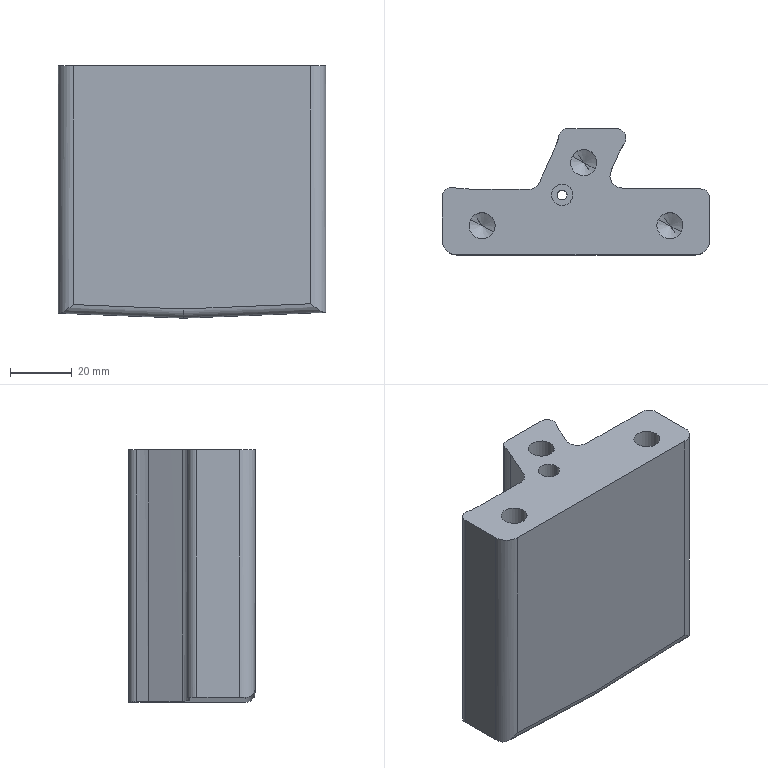Part | CATIA | 1 solid | 42 faces | box 87 x 41 x 82 mm | volume 179725 mm3 | cylinder 27 | plane 9 | cone 6 | commonest cylinder face diameters 6 x6 8.5 x6 40 x4 3.2 x2 7 x2 8 x2
STEP:
#1=CARTESIAN_POINT('',(-189.,-29.5,41.546));
#2=VERTEX_POINT('',#1);
#3=CARTESIAN_POINT('',(-192.73,-27.462,44.));
#4=VERTEX_POINT('',#3);
#5=CARTESIAN_POINT('',(-190.865,-28.481,42.773));
#6=DIRECTION('',(-0.76,0.4152,0.5));
#7=VECTOR('',#6,1.);
#8=LINE('',#5,#7);
#9=EDGE_CURVE('',#2,#4,#8,.T.);
#10=ORIENTED_EDGE('',*,*,#9,.T.);
#11=CARTESIAN_POINT('',(-185.27,-31.538,44.));
#12=VERTEX_POINT('',#11);
#13=CARTESIAN_POINT('',(-189.,-29.5,44.));
#14=DIRECTION('',(0.,0.,1.));
#15=AXIS2_PLACEMENT_3D('',#13,#14,$);
#16=CIRCLE('',#15,4.25);
#17=EDGE_CURVE('',#12,#4,#16,.F.);
#18=ORIENTED_EDGE('',*,*,#17,.F.);
#19=CARTESIAN_POINT('',(-187.135,-30.519,42.773));
#20=DIRECTION('',(0.76,-0.4152,0.5));
#21=VECTOR('',#20,1.);
#22=LINE('',#19,#21);
#23=EDGE_CURVE('',#2,#12,#22,.T.);
#24=ORIENTED_EDGE('',*,*,#23,.F.);
#25=EDGE_LOOP('',(#10,#18,#24));
#26=FACE_OUTER_BOUND('',#25,.T.);
#27=CARTESIAN_POINT('',(-189.,-29.5,41.546));
#28=DIRECTION('',(0.,0.,1.));
#29=DIRECTION('',(0.8776,-0.4794,0.));
#30=AXIS2_PLACEMENT_3D('',#27,#28,#29);
#31=CONICAL_SURFACE('',#30,0.,1.047);
#32=ADVANCED_FACE('',(#26),#31,.F.);
#33=ORIENTED_EDGE('',*,*,#23,.T.);
#34=CARTESIAN_POINT('',(-189.,-29.5,44.));
#35=DIRECTION('',(0.,0.,1.));
#36=AXIS2_PLACEMENT_3D('',#34,#35,$);
#37=CIRCLE('',#36,4.25);
#38=EDGE_CURVE('',#4,#12,#37,.F.);
#39=ORIENTED_EDGE('',*,*,#38,.F.);
#40=ORIENTED_EDGE('',*,*,#9,.F.);
#41=EDGE_LOOP('',(#33,#39,#40));
#42=FACE_OUTER_BOUND('',#41,.T.);
#43=ADVANCED_FACE('',(#42),#31,.F.);
#44=CARTESIAN_POINT('',(-192.73,-27.462,69.));
#45=VERTEX_POINT('',#44);
#46=CARTESIAN_POINT('',(-185.27,-31.538,69.));
#47=VERTEX_POINT('',#46);
#48=CARTESIAN_POINT('',(-189.,-29.5,69.));
#49=DIRECTION('',(0.,0.,-1.));
#50=AXIS2_PLACEMENT_3D('',#48,#49,$);
#51=CIRCLE('',#50,4.25);
#52=EDGE_CURVE('',#45,#47,#51,.F.);
#53=ORIENTED_EDGE('',*,*,#52,.T.);
#54=CARTESIAN_POINT('',(-185.27,-31.538,56.655));
#55=DIRECTION('',(0.,0.,-1.));
#56=VECTOR('',#55,1.);
#57=LINE('',#54,#56);
#58=EDGE_CURVE('',#12,#47,#57,.F.);
#59=ORIENTED_EDGE('',*,*,#58,.F.);
#60=ORIENTED_EDGE('',*,*,#17,.T.);
#61=CARTESIAN_POINT('',(-192.73,-27.462,56.655));
#62=DIRECTION('',(0.,0.,-1.));
#63=VECTOR('',#62,1.);
#64=LINE('',#61,#63);
#65=EDGE_CURVE('',#4,#45,#64,.F.);
#66=ORIENTED_EDGE('',*,*,#65,.T.);
#67=EDGE_LOOP('',(#53,#59,#60,#66));
#68=FACE_OUTER_BOUND('',#67,.T.);
#69=CARTESIAN_POINT('',(-189.,-29.5,68.9));
#70=DIRECTION('',(0.,0.,-1.));
#71=DIRECTION('',(0.8776,-0.4794,0.));
#72=AXIS2_PLACEMENT_3D('',#69,#70,#71);
#73=CYLINDRICAL_SURFACE('',#72,4.25);
#74=ADVANCED_FACE('',(#68),#73,.F.);
#75=CARTESIAN_POINT('',(-189.,-29.5,69.));
#76=DIRECTION('',(0.,0.,-1.));
#77=AXIS2_PLACEMENT_3D('',#75,#76,$);
#78=CIRCLE('',#77,4.25);
#79=EDGE_CURVE('',#47,#45,#78,.F.);
#80=ORIENTED_EDGE('',*,*,#79,.T.);
#81=ORIENTED_EDGE('',*,*,#65,.F.);
#82=ORIENTED_EDGE('',*,*,#38,.T.);
#83=ORIENTED_EDGE('',*,*,#58,.T.);
#84=EDGE_LOOP('',(#80,#81,#82,#83));
#85=FACE_OUTER_BOUND('',#84,.T.);
#86=ADVANCED_FACE('',(#85),#73,.F.);
#87=CARTESIAN_POINT('',(-161.,-50.,41.546));
#88=VERTEX_POINT('',#87);
#89=CARTESIAN_POINT('',(-164.73,-47.962,44.));
#90=VERTEX_POINT('',#89);
#91=CARTESIAN_POINT('',(-162.865,-48.981,42.773));
#92=DIRECTION('',(-0.76,0.4152,0.5));
#93=VECTOR('',#92,1.);
#94=LINE('',#91,#93);
#95=EDGE_CURVE('',#88,#90,#94,.T.);
#96=ORIENTED_EDGE('',*,*,#95,.T.);
#97=CARTESIAN_POINT('',(-157.27,-52.038,44.));
#98=VERTEX_POINT('',#97);
#99=CARTESIAN_POINT('',(-161.,-50.,44.));
#100=DIRECTION('',(0.,0.,1.));
#101=AXIS2_PLACEMENT_3D('',#99,#100,$);
#102=CIRCLE('',#101,4.25);
#103=EDGE_CURVE('',#98,#90,#102,.F.);
#104=ORIENTED_EDGE('',*,*,#103,.F.);
#105=CARTESIAN_POINT('',(-159.135,-51.019,42.773));
#106=DIRECTION('',(0.76,-0.4152,0.5));
#107=VECTOR('',#106,1.);
#108=LINE('',#105,#107);
#109=EDGE_CURVE('',#88,#98,#108,.T.);
#110=ORIENTED_EDGE('',*,*,#109,.F.);
#111=EDGE_LOOP('',(#96,#104,#110));
#112=FACE_OUTER_BOUND('',#111,.T.);
#113=CARTESIAN_POINT('',(-161.,-50.,41.546));
#114=DIRECTION('',(0.,0.,1.));
#115=DIRECTION('',(0.8776,-0.4794,0.));
#116=AXIS2_PLACEMENT_3D('',#113,#114,#115);
#117=CONICAL_SURFACE('',#116,0.,1.047);
#118=ADVANCED_FACE('',(#112),#117,.F.);
#119=ORIENTED_EDGE('',*,*,#109,.T.);
#120=CARTESIAN_POINT('',(-161.,-50.,44.));
#121=DIRECTION('',(0.,0.,1.));
#122=AXIS2_PLACEMENT_3D('',#120,#121,$);
#123=CIRCLE('',#122,4.25);
#124=EDGE_CURVE('',#90,#98,#123,.F.);
#125=ORIENTED_EDGE('',*,*,#124,.F.);
#126=ORIENTED_EDGE('',*,*,#95,.F.);
#127=EDGE_LOOP('',(#119,#125,#126));
#128=FACE_OUTER_BOUND('',#127,.T.);
#129=ADVANCED_FACE('',(#128),#117,.F.);
#130=CARTESIAN_POINT('',(-164.73,-47.962,69.));
#131=VERTEX_POINT('',#130);
#132=CARTESIAN_POINT('',(-157.27,-52.038,69.));
#133=VERTEX_POINT('',#132);
#134=CARTESIAN_POINT('',(-161.,-50.,69.));
#135=DIRECTION('',(0.,0.,-1.));
#136=AXIS2_PLACEMENT_3D('',#134,#135,$);
#137=CIRCLE('',#136,4.25);
#138=EDGE_CURVE('',#131,#133,#137,.F.);
#139=ORIENTED_EDGE('',*,*,#138,.T.);
#140=CARTESIAN_POINT('',(-157.27,-52.038,56.655));
#141=DIRECTION('',(0.,0.,-1.));
#142=VECTOR('',#141,1.);
#143=LINE('',#140,#142);
#144=EDGE_CURVE('',#98,#133,#143,.F.);
#145=ORIENTED_EDGE('',*,*,#144,.F.);
#146=ORIENTED_EDGE('',*,*,#103,.T.);
#147=CARTESIAN_POINT('',(-164.73,-47.962,56.655));
#148=DIRECTION('',(0.,0.,-1.));
#149=VECTOR('',#148,1.);
#150=LINE('',#147,#149);
#151=EDGE_CURVE('',#90,#131,#150,.F.);
#152=ORIENTED_EDGE('',*,*,#151,.T.);
#153=EDGE_LOOP('',(#139,#145,#146,#152));
#154=FACE_OUTER_BOUND('',#153,.T.);
#155=CARTESIAN_POINT('',(-161.,-50.,68.9));
#156=DIRECTION('',(0.,0.,-1.));
#157=DIRECTION('',(0.8776,-0.4794,0.));
#158=AXIS2_PLACEMENT_3D('',#155,#156,#157);
#159=CYLINDRICAL_SURFACE('',#158,4.25);
#160=ADVANCED_FACE('',(#154),#159,.F.);
#161=CARTESIAN_POINT('',(-161.,-50.,69.));
#162=DIRECTION('',(0.,0.,-1.));
#163=AXIS2_PLACEMENT_3D('',#161,#162,$);
#164=CIRCLE('',#163,4.25);
#165=EDGE_CURVE('',#133,#131,#164,.F.);
#166=ORIENTED_EDGE('',*,*,#165,.T.);
#167=ORIENTED_EDGE('',*,*,#151,.F.);
#168=ORIENTED_EDGE('',*,*,#124,.T.);
#169=ORIENTED_EDGE('',*,*,#144,.T.);
#170=EDGE_LOOP('',(#166,#167,#168,#169));
#171=FACE_OUTER_BOUND('',#170,.T.);
#172=ADVANCED_FACE('',(#171),#159,.F.);
#173=CARTESIAN_POINT('',(-222.,-50.,41.546));
#174=VERTEX_POINT('',#173);
#175=CARTESIAN_POINT('',(-225.73,-47.962,44.));
#176=VERTEX_POINT('',#175);
#177=CARTESIAN_POINT('',(-223.865,-48.981,42.773));
#178=DIRECTION('',(-0.76,0.4152,0.5));
#179=VECTOR('',#178,1.);
#180=LINE('',#177,#179);
#181=EDGE_CURVE('',#174,#176,#180,.T.);
#182=ORIENTED_EDGE('',*,*,#181,.T.);
#183=CARTESIAN_POINT('',(-218.27,-52.038,44.));
#184=VERTEX_POINT('',#183);
#185=CARTESIAN_POINT('',(-222.,-50.,44.));
#186=DIRECTION('',(0.,0.,1.));
#187=AXIS2_PLACEMENT_3D('',#185,#186,$);
#188=CIRCLE('',#187,4.25);
#189=EDGE_CURVE('',#184,#176,#188,.F.);
#190=ORIENTED_EDGE('',*,*,#189,.F.);
#191=CARTESIAN_POINT('',(-220.135,-51.019,42.773));
#192=DIRECTION('',(0.76,-0.4152,0.5));
#193=VECTOR('',#192,1.);
#194=LINE('',#191,#193);
#195=EDGE_CURVE('',#174,#184,#194,.T.);
#196=ORIENTED_EDGE('',*,*,#195,.F.);
#197=EDGE_LOOP('',(#182,#190,#196));
#198=FACE_OUTER_BOUND('',#197,.T.);
#199=CARTESIAN_POINT('',(-222.,-50.,41.546));
#200=DIRECTION('',(0.,0.,1.));
#201=DIRECTION('',(0.8776,-0.4794,0.));
#202=AXIS2_PLACEMENT_3D('',#199,#200,#201);
#203=CONICAL_SURFACE('',#202,0.,1.047);
#204=ADVANCED_FACE('',(#198),#203,.F.);
#205=ORIENTED_EDGE('',*,*,#195,.T.);
#206=CARTESIAN_POINT('',(-222.,-50.,44.));
#207=DIRECTION('',(0.,0.,1.));
#208=AXIS2_PLACEMENT_3D('',#206,#207,$);
#209=CIRCLE('',#208,4.25);
#210=EDGE_CURVE('',#176,#184,#209,.F.);
#211=ORIENTED_EDGE('',*,*,#210,.F.);
#212=ORIENTED_EDGE('',*,*,#181,.F.);
#213=EDGE_LOOP('',(#205,#211,#212));
#214=FACE_OUTER_BOUND('',#213,.T.);
#215=ADVANCED_FACE('',(#214),#203,.F.);
#216=CARTESIAN_POINT('',(-225.73,-47.962,69.));
#217=VERTEX_POINT('',#216);
#218=CARTESIAN_POINT('',(-218.27,-52.038,69.));
#219=VERTEX_POINT('',#218);
#220=CARTESIAN_POINT('',(-222.,-50.,69.));
#221=DIRECTION('',(0.,0.,-1.));
#222=AXIS2_PLACEMENT_3D('',#220,#221,$);
#223=CIRCLE('',#222,4.25);
#224=EDGE_CURVE('',#217,#219,#223,.F.);
#225=ORIENTED_EDGE('',*,*,#224,.T.);
#226=CARTESIAN_POINT('',(-218.27,-52.038,56.655));
#227=DIRECTION('',(0.,0.,-1.));
#228=VECTOR('',#227,1.);
#229=LINE('',#226,#228);
#230=EDGE_CURVE('',#184,#219,#229,.F.);
#231=ORIENTED_EDGE('',*,*,#230,.F.);
#232=ORIENTED_EDGE('',*,*,#189,.T.);
#233=CARTESIAN_POINT('',(-225.73,-47.962,56.655));
#234=DIRECTION('',(0.,0.,-1.));
#235=VECTOR('',#234,1.);
#236=LINE('',#233,#235);
#237=EDGE_CURVE('',#176,#217,#236,.F.);
#238=ORIENTED_EDGE('',*,*,#237,.T.);
#239=EDGE_LOOP('',(#225,#231,#232,#238));
#240=FACE_OUTER_BOUND('',#239,.T.);
#241=CARTESIAN_POINT('',(-222.,-50.,68.9));
#242=DIRECTION('',(0.,0.,-1.));
#243=DIRECTION('',(0.8776,-0.4794,0.));
#244=AXIS2_PLACEMENT_3D('',#241,#242,#243);
#245=CYLINDRICAL_SURFACE('',#244,4.25);
#246=ADVANCED_FACE('',(#240),#245,.F.);
#247=CARTESIAN_POINT('',(-222.,-50.,69.));
#248=DIRECTION('',(0.,0.,-1.));
#249=AXIS2_PLACEMENT_3D('',#247,#248,$);
#250=CIRCLE('',#249,4.25);
#251=EDGE_CURVE('',#219,#217,#250,.F.);
#252=ORIENTED_EDGE('',*,*,#251,.T.);
#253=ORIENTED_EDGE('',*,*,#237,.F.);
#254=ORIENTED_EDGE('',*,*,#210,.T.);
#255=ORIENTED_EDGE('',*,*,#230,.T.);
#256=EDGE_LOOP('',(#252,#253,#254,#255));
#257=FACE_OUTER_BOUND('',#256,.T.);
#258=ADVANCED_FACE('',(#257),#245,.F.);
#259=CARTESIAN_POINT('',(-177.609,-26.493,-12.327));
#260=VERTEX_POINT('',#259);
#261=CARTESIAN_POINT('',(-177.609,-26.493,69.));
#262=VERTEX_POINT('',#261);
#263=CARTESIAN_POINT('',(-177.609,-26.493,28.61));
#264=DIRECTION('',(0.,0.,1.));
#265=VECTOR('',#264,1.);
#266=LINE('',#263,#265);
#267=EDGE_CURVE('',#260,#262,#266,.T.);
#268=ORIENTED_EDGE('',*,*,#267,.T.);
#269=CARTESIAN_POINT('',(-177.721,-26.749,69.));
#270=VERTEX_POINT('',#269);
#271=CARTESIAN_POINT('',(-195.994,-18.618,69.));
#272=DIRECTION('',(0.,0.,1.));
#273=AXIS2_PLACEMENT_3D('',#271,#272,$);
#274=CIRCLE('',#273,20.);
#275=EDGE_CURVE('',#270,#262,#274,.T.);
#276=ORIENTED_EDGE('',*,*,#275,.F.);
#277=CARTESIAN_POINT('',(-177.721,-26.749,-12.332));
#278=VERTEX_POINT('',#277);
#279=CARTESIAN_POINT('',(-177.721,-26.749,28.61));
#280=DIRECTION('',(0.,0.,1.));
#281=VECTOR('',#280,1.);
#282=LINE('',#279,#281);
#283=EDGE_CURVE('',#278,#270,#282,.T.);
#284=ORIENTED_EDGE('',*,*,#283,.F.);
#285=CARTESIAN_POINT('',(-177.609,-26.493,-12.327));
#286=CARTESIAN_POINT('',(-177.646,-26.579,-12.329));
#287=CARTESIAN_POINT('',(-177.683,-26.664,-12.33));
#288=CARTESIAN_POINT('',(-177.721,-26.749,-12.332));
#289=B_SPLINE_CURVE_WITH_KNOTS('',3,(#285,#286,#287,#288),.UNSPECIFIED.,.F.,.U.,(4,4),(0.,0.3946),.UNSPECIFIED.);
#290=EDGE_CURVE('',#260,#278,#289,.T.);
#291=ORIENTED_EDGE('',*,*,#290,.F.);
#292=EDGE_LOOP('',(#268,#276,#284,#291));
#293=FACE_OUTER_BOUND('',#292,.T.);
#294=CARTESIAN_POINT('',(-195.994,-18.618,28.61));
#295=DIRECTION('',(0.,0.,1.));
#296=DIRECTION('',(0.9136,-0.4065,0.));
#297=AXIS2_PLACEMENT_3D('',#294,#295,#296);
#298=CYLINDRICAL_SURFACE('',#297,20.);
#299=ADVANCED_FACE('',(#293),#298,.T.);
#300=CARTESIAN_POINT('',(-175.802,-23.179,-12.254));
#301=VERTEX_POINT('',#300);
#302=CARTESIAN_POINT('',(-177.609,-26.493,-12.327));
#303=CARTESIAN_POINT('',(-177.113,-25.335,-12.307));
#304=CARTESIAN_POINT('',(-176.507,-24.223,-12.282));
#305=CARTESIAN_POINT('',(-175.802,-23.179,-12.254));
#306=B_SPLINE_CURVE_WITH_KNOTS('',3,(#302,#303,#304,#305),.UNSPECIFIED.,.F.,.U.,(4,4),(0.,5.349),.UNSPECIFIED.);
#307=EDGE_CURVE('',#260,#301,#306,.T.);
#308=ORIENTED_EDGE('',*,*,#307,.T.);
#309=CARTESIAN_POINT('',(-175.802,-23.179,69.));
#310=VERTEX_POINT('',#309);
#311=CARTESIAN_POINT('',(-175.802,-23.179,28.61));
#312=DIRECTION('',(0.,0.,1.));
#313=VECTOR('',#312,1.);
#314=LINE('',#311,#313);
#315=EDGE_CURVE('',#301,#310,#314,.T.);
#316=ORIENTED_EDGE('',*,*,#315,.T.);
#317=CARTESIAN_POINT('',(-159.225,-34.369,69.));
#318=DIRECTION('',(0.,0.,1.));
#319=AXIS2_PLACEMENT_3D('',#317,#318,$);
#320=CIRCLE('',#319,20.);
#321=EDGE_CURVE('',#310,#262,#320,.T.);
#322=ORIENTED_EDGE('',*,*,#321,.T.);
#323=ORIENTED_EDGE('',*,*,#267,.F.);
#324=EDGE_LOOP('',(#308,#316,#322,#323));
#325=FACE_OUTER_BOUND('',#324,.T.);
#326=CARTESIAN_POINT('',(-159.225,-34.369,28.61));
#327=DIRECTION('',(0.,0.,1.));
#328=DIRECTION('',(-0.8288,0.5595,0.));
#329=AXIS2_PLACEMENT_3D('',#326,#327,#328);
#330=CYLINDRICAL_SURFACE('',#329,20.);
#331=ADVANCED_FACE('',(#325),#330,.F.);
#332=CARTESIAN_POINT('',(-178.288,-18.5,-12.355));
#333=VERTEX_POINT('',#332);
#334=CARTESIAN_POINT('',(-178.288,-18.5,69.));
#335=VERTEX_POINT('',#334);
#336=CARTESIAN_POINT('',(-178.288,-18.5,28.61));
#337=DIRECTION('',(0.,0.,1.));
#338=VECTOR('',#337,1.);
#339=LINE('',#336,#338);
#340=EDGE_CURVE('',#333,#335,#339,.T.);
#341=ORIENTED_EDGE('',*,*,#340,.T.);
#342=CARTESIAN_POINT('',(-178.288,-21.5,69.));
#343=DIRECTION('',(0.,0.,1.));
#344=AXIS2_PLACEMENT_3D('',#342,#343,$);
#345=CIRCLE('',#344,3.);
#346=EDGE_CURVE('',#310,#335,#345,.T.);
#347=ORIENTED_EDGE('',*,*,#346,.F.);
#348=ORIENTED_EDGE('',*,*,#315,.F.);
#349=CARTESIAN_POINT('',(-175.802,-23.179,-12.254));
#350=CARTESIAN_POINT('',(-175.075,-22.102,-12.224));
#351=CARTESIAN_POINT('',(-174.922,-20.628,-12.218));
#352=CARTESIAN_POINT('',(-175.685,-19.196,-12.249));
#353=CARTESIAN_POINT('',(-176.99,-18.5,-12.302));
#354=CARTESIAN_POINT('',(-178.288,-18.5,-12.355));
#355=B_SPLINE_CURVE_WITH_KNOTS('',5,(#349,#350,#351,#352,#353,#354),.UNSPECIFIED.,.F.,.U.,(6,6),(0.,9.186),.UNSPECIFIED.);
#356=EDGE_CURVE('',#301,#333,#355,.T.);
#357=ORIENTED_EDGE('',*,*,#356,.T.);
#358=EDGE_LOOP('',(#341,#347,#348,#357));
#359=FACE_OUTER_BOUND('',#358,.T.);
#360=CARTESIAN_POINT('',(-178.288,-21.5,28.61));
#361=DIRECTION('',(0.,0.,1.));
#362=DIRECTION('',(0.8288,-0.5595,0.));
#363=AXIS2_PLACEMENT_3D('',#360,#361,#362);
#364=CYLINDRICAL_SURFACE('',#363,3.);
#365=ADVANCED_FACE('',(#359),#364,.T.);
#366=CARTESIAN_POINT('',(-194.142,-18.5,-13.));
#367=VERTEX_POINT('',#366);
#368=CARTESIAN_POINT('',(-194.142,-18.5,69.));
#369=VERTEX_POINT('',#368);
#370=CARTESIAN_POINT('',(-194.142,-18.5,28.));
#371=DIRECTION('',(0.,0.,1.));
#372=VECTOR('',#371,1.);
#373=LINE('',#370,#372);
#374=EDGE_CURVE('',#367,#369,#373,.T.);
#375=ORIENTED_EDGE('',*,*,#374,.T.);
#376=CARTESIAN_POINT('',(-186.215,-18.5,69.));
#377=DIRECTION('',(-1.,0.,0.));
#378=VECTOR('',#377,1.);
#379=LINE('',#376,#378);
#380=EDGE_CURVE('',#335,#369,#379,.T.);
#381=ORIENTED_EDGE('',*,*,#380,.F.);
#382=ORIENTED_EDGE('',*,*,#340,.F.);
#383=CARTESIAN_POINT('',(-186.215,-18.5,-12.677));
#384=DIRECTION('',(0.9992,0.,0.04066));
#385=VECTOR('',#384,1.);
#386=LINE('',#383,#385);
#387=EDGE_CURVE('',#367,#333,#386,.T.);
#388=ORIENTED_EDGE('',*,*,#387,.F.);
#389=EDGE_LOOP('',(#375,#381,#382,#388));
#390=FACE_OUTER_BOUND('',#389,.T.);
#391=CARTESIAN_POINT('',(-178.288,-18.5,0.));
#392=DIRECTION('',(0.,1.,0.));
#393=DIRECTION('',(-1.,0.,0.));
#394=AXIS2_PLACEMENT_3D('',#391,#392,#393);
#395=PLANE('',#394);
#396=ADVANCED_FACE('',(#390),#395,.T.);
#397=CARTESIAN_POINT('',(-197.075,-20.866,-12.885));
#398=VERTEX_POINT('',#397);
#399=CARTESIAN_POINT('',(-197.075,-20.866,69.));
#400=VERTEX_POINT('',#399);
#401=CARTESIAN_POINT('',(-197.075,-20.866,28.61));
#402=DIRECTION('',(0.,0.,1.));
#403=VECTOR('',#402,1.);
#404=LINE('',#401,#403);
#405=EDGE_CURVE('',#398,#400,#404,.T.);
#406=ORIENTED_EDGE('',*,*,#405,.T.);
#407=CARTESIAN_POINT('',(-194.142,-21.5,69.));
#408=DIRECTION('',(0.,0.,1.));
#409=AXIS2_PLACEMENT_3D('',#407,#408,$);
#410=CIRCLE('',#409,3.);
#411=EDGE_CURVE('',#369,#400,#410,.T.);
#412=ORIENTED_EDGE('',*,*,#411,.F.);
#413=ORIENTED_EDGE('',*,*,#374,.F.);
#414=CARTESIAN_POINT('',(-197.075,-20.866,-12.885));
#415=CARTESIAN_POINT('',(-196.902,-20.069,-12.891));
#416=CARTESIAN_POINT('',(-196.46,-19.331,-12.909));
#417=CARTESIAN_POINT('',(-195.772,-18.776,-12.936));
#418=CARTESIAN_POINT('',(-194.957,-18.5,-12.968));
#419=CARTESIAN_POINT('',(-194.142,-18.5,-13.));
#420=B_SPLINE_CURVE_WITH_KNOTS('',5,(#414,#415,#416,#417,#418,#419),.UNSPECIFIED.,.F.,.U.,(6,6),(0.,5.763),.UNSPECIFIED.);
#421=EDGE_CURVE('',#398,#367,#420,.T.);
#422=ORIENTED_EDGE('',*,*,#421,.F.);
#423=EDGE_LOOP('',(#406,#412,#413,#422));
#424=FACE_OUTER_BOUND('',#423,.T.);
#425=CARTESIAN_POINT('',(-194.142,-21.5,28.61));
#426=DIRECTION('',(0.,0.,1.));
#427=DIRECTION('',(0.,1.,0.));
#428=AXIS2_PLACEMENT_3D('',#425,#426,#427);
#429=CYLINDRICAL_SURFACE('',#428,3.);
#430=ADVANCED_FACE('',(#424),#429,.T.);
#431=CARTESIAN_POINT('',(-198.375,-24.825,-12.834));
#432=VERTEX_POINT('',#431);
#433=CARTESIAN_POINT('',(-197.075,-20.866,-12.885));
#434=CARTESIAN_POINT('',(-197.369,-22.226,-12.873));
#435=CARTESIAN_POINT('',(-197.805,-23.555,-12.856));
#436=CARTESIAN_POINT('',(-198.375,-24.825,-12.834));
#437=B_SPLINE_CURVE_WITH_KNOTS('',3,(#433,#434,#435,#436),.UNSPECIFIED.,.F.,.U.,(4,4),(0.,5.904),.UNSPECIFIED.);
#438=EDGE_CURVE('',#398,#432,#437,.T.);
#439=ORIENTED_EDGE('',*,*,#438,.T.);
#440=CARTESIAN_POINT('',(-198.375,-24.825,69.));
#441=VERTEX_POINT('',#440);
#442=CARTESIAN_POINT('',(-198.375,-24.825,28.61));
#443=DIRECTION('',(0.,0.,1.));
#444=VECTOR('',#443,1.);
#445=LINE('',#442,#444);
#446=EDGE_CURVE('',#432,#441,#445,.T.);
#447=ORIENTED_EDGE('',*,*,#446,.T.);
#448=CARTESIAN_POINT('',(-216.623,-16.639,69.));
#449=DIRECTION('',(0.,0.,1.));
#450=AXIS2_PLACEMENT_3D('',#448,#449,$);
#451=CIRCLE('',#450,20.);
#452=EDGE_CURVE('',#441,#400,#451,.T.);
#453=ORIENTED_EDGE('',*,*,#452,.T.);
#454=ORIENTED_EDGE('',*,*,#405,.F.);
#455=EDGE_LOOP('',(#439,#447,#453,#454));
#456=FACE_OUTER_BOUND('',#455,.T.);
#457=CARTESIAN_POINT('',(-216.623,-16.639,28.61));
#458=DIRECTION('',(0.,0.,1.));
#459=DIRECTION('',(0.9124,-0.4093,0.));
#460=AXIS2_PLACEMENT_3D('',#457,#458,#459);
#461=CYLINDRICAL_SURFACE('',#460,20.);
#462=ADVANCED_FACE('',(#456),#461,.F.);
#463=CARTESIAN_POINT('',(-203.323,-35.871,-12.639));
#464=VERTEX_POINT('',#463);
#465=CARTESIAN_POINT('',(-203.323,-35.871,69.));
#466=VERTEX_POINT('',#465);
#467=CARTESIAN_POINT('',(-203.323,-35.871,28.61));
#468=DIRECTION('',(0.,0.,1.));
#469=VECTOR('',#468,1.);
#470=LINE('',#467,#469);
#471=EDGE_CURVE('',#464,#466,#470,.T.);
#472=ORIENTED_EDGE('',*,*,#471,.T.);
#473=CARTESIAN_POINT('',(11407.219,-5230.648,69.));
#474=DIRECTION('',(0.,0.,1.));
#475=AXIS2_PLACEMENT_3D('',#473,#474,$);
#476=CIRCLE('',#475,12719.686);
#477=EDGE_CURVE('',#441,#466,#476,.T.);
#478=ORIENTED_EDGE('',*,*,#477,.F.);
#479=ORIENTED_EDGE('',*,*,#446,.F.);
#480=CARTESIAN_POINT('',(-203.323,-35.871,-12.639));
#481=CARTESIAN_POINT('',(-201.675,-32.188,-12.704));
#482=CARTESIAN_POINT('',(-200.026,-28.506,-12.769));
#483=CARTESIAN_POINT('',(-198.375,-24.825,-12.834));
#484=B_SPLINE_CURVE_WITH_KNOTS('',3,(#480,#481,#482,#483),.UNSPECIFIED.,.F.,.U.,(4,4),(0.,17.12),.UNSPECIFIED.);
#485=EDGE_CURVE('',#464,#432,#484,.T.);
#486=ORIENTED_EDGE('',*,*,#485,.F.);
#487=EDGE_LOOP('',(#472,#478,#479,#486));
#488=FACE_OUTER_BOUND('',#487,.T.);
#489=CARTESIAN_POINT('',(11407.219,-5230.648,28.61));
#490=DIRECTION('',(0.,0.,1.));
#491=DIRECTION('',(-0.9124,0.4093,0.));
#492=AXIS2_PLACEMENT_3D('',#489,#490,#491);
#493=CYLINDRICAL_SURFACE('',#492,12719.686);
#494=ADVANCED_FACE('',(#488),#493,.T.);
#495=CARTESIAN_POINT('',(-206.999,-38.237,-12.494));
#496=VERTEX_POINT('',#495);
#497=CARTESIAN_POINT('',(-203.323,-35.871,-12.639));
#498=CARTESIAN_POINT('',(-203.796,-36.926,-12.62));
#499=CARTESIAN_POINT('',(-204.679,-37.803,-12.586));
#500=CARTESIAN_POINT('',(-205.843,-38.244,-12.54));
#501=CARTESIAN_POINT('',(-206.999,-38.237,-12.494));
#502=B_SPLINE_CURVE_WITH_KNOTS('',4,(#497,#498,#499,#500,#501),.UNSPECIFIED.,.F.,.U.,(5,5),(0.,6.544),.UNSPECIFIED.);
#503=EDGE_CURVE('',#464,#496,#502,.T.);
#504=ORIENTED_EDGE('',*,*,#503,.T.);
#505=CARTESIAN_POINT('',(-206.999,-38.237,69.));
#506=VERTEX_POINT('',#505);
#507=CARTESIAN_POINT('',(-206.999,-38.237,28.61));
#508=DIRECTION('',(0.,0.,1.));
#509=VECTOR('',#508,1.);
#510=LINE('',#507,#509);
#511=EDGE_CURVE('',#496,#506,#510,.T.);
#512=ORIENTED_EDGE('',*,*,#511,.T.);
#513=CARTESIAN_POINT('',(-206.974,-34.237,69.));
#514=DIRECTION('',(0.,0.,1.));
#515=AXIS2_PLACEMENT_3D('',#513,#514,$);
#516=CIRCLE('',#515,4.);
#517=EDGE_CURVE('',#506,#466,#516,.T.);
#518=ORIENTED_EDGE('',*,*,#517,.T.);
#519=ORIENTED_EDGE('',*,*,#471,.F.);
#520=EDGE_LOOP('',(#504,#512,#518,#519));
#521=FACE_OUTER_BOUND('',#520,.T.);
#522=CARTESIAN_POINT('',(-206.974,-34.237,28.61));
#523=DIRECTION('',(0.,0.,1.));
#524=DIRECTION('',(-0.006107,-1.,0.));
#525=AXIS2_PLACEMENT_3D('',#522,#523,#524);
#526=CYLINDRICAL_SURFACE('',#525,4.);
#527=ADVANCED_FACE('',(#521),#526,.F.);
#528=CARTESIAN_POINT('',(-227.202,-38.088,-11.7));
#529=VERTEX_POINT('',#528);
#530=CARTESIAN_POINT('',(-227.202,-38.088,-11.7));
#531=CARTESIAN_POINT('',(-220.468,-38.146,-11.965));
#532=CARTESIAN_POINT('',(-213.733,-38.196,-12.23));
#533=CARTESIAN_POINT('',(-206.999,-38.237,-12.494));
#534=B_SPLINE_CURVE_WITH_KNOTS('',3,(#530,#531,#532,#533),.UNSPECIFIED.,.F.,.U.,(4,4),(0.,28.595),.UNSPECIFIED.);
#535=EDGE_CURVE('',#529,#496,#534,.T.);
#536=ORIENTED_EDGE('',*,*,#535,.F.);
#537=CARTESIAN_POINT('',(-227.202,-38.088,69.));
#538=VERTEX_POINT('',#537);
#539=CARTESIAN_POINT('',(-227.202,-38.088,28.61));
#540=DIRECTION('',(0.,0.,1.));
#541=VECTOR('',#540,1.);
#542=LINE('',#539,#541);
#543=EDGE_CURVE('',#529,#538,#542,.T.);
#544=ORIENTED_EDGE('',*,*,#543,.T.);
#545=CARTESIAN_POINT('',(-158.792,7855.513,69.));
#546=DIRECTION('',(0.,0.,1.));
#547=AXIS2_PLACEMENT_3D('',#545,#546,$);
#548=CIRCLE('',#547,7893.897);
#549=EDGE_CURVE('',#538,#506,#548,.T.);
#550=ORIENTED_EDGE('',*,*,#549,.T.);
#551=ORIENTED_EDGE('',*,*,#511,.F.);
#552=EDGE_LOOP('',(#536,#544,#550,#551));
#553=FACE_OUTER_BOUND('',#552,.T.);
#554=CARTESIAN_POINT('',(-158.792,7855.513,28.61));
#555=DIRECTION('',(0.,0.,1.));
#556=DIRECTION('',(-0.008666,-1.,0.));
#557=AXIS2_PLACEMENT_3D('',#554,#555,#556);
#558=CYLINDRICAL_SURFACE('',#557,7893.897);
#559=ADVANCED_FACE('',(#553),#558,.F.);
#560=CARTESIAN_POINT('',(-231.352,-37.616,-11.537));
#561=VERTEX_POINT('',#560);
#562=CARTESIAN_POINT('',(-231.352,-37.616,-11.537));
#563=CARTESIAN_POINT('',(-229.99,-37.917,-11.59));
#564=CARTESIAN_POINT('',(-228.597,-38.076,-11.645));
#565=CARTESIAN_POINT('',(-227.202,-38.088,-11.7));
#566=B_SPLINE_CURVE_WITH_KNOTS('',3,(#562,#563,#564,#565),.UNSPECIFIED.,.F.,.U.,(4,4),(0.,5.921),.UNSPECIFIED.);
#567=EDGE_CURVE('',#561,#529,#566,.T.);
#568=ORIENTED_EDGE('',*,*,#567,.F.);
#569=CARTESIAN_POINT('',(-231.352,-37.616,69.));
#570=VERTEX_POINT('',#569);
#571=CARTESIAN_POINT('',(-231.352,-37.616,28.61));
#572=DIRECTION('',(0.,0.,1.));
#573=VECTOR('',#572,1.);
#574=LINE('',#571,#573);
#575=EDGE_CURVE('',#561,#570,#574,.T.);
#576=ORIENTED_EDGE('',*,*,#575,.T.);
#577=CARTESIAN_POINT('',(-227.029,-18.088,69.));
#578=DIRECTION('',(0.,0.,1.));
#579=AXIS2_PLACEMENT_3D('',#577,#578,$);
#580=CIRCLE('',#579,20.);
#581=EDGE_CURVE('',#570,#538,#580,.T.);
#582=ORIENTED_EDGE('',*,*,#581,.T.);
#583=ORIENTED_EDGE('',*,*,#543,.F.);
#584=EDGE_LOOP('',(#568,#576,#582,#583));
#585=FACE_OUTER_BOUND('',#584,.T.);
#586=CARTESIAN_POINT('',(-227.029,-18.088,28.61));
#587=DIRECTION('',(0.,0.,1.));
#588=DIRECTION('',(-0.2161,-0.9764,0.));
#589=AXIS2_PLACEMENT_3D('',#586,#587,#588);
#590=CYLINDRICAL_SURFACE('',#589,20.);
#591=ADVANCED_FACE('',(#585),#590,.F.);
#592=CARTESIAN_POINT('',(-235.,-40.545,-11.393));
#593=VERTEX_POINT('',#592);
#594=CARTESIAN_POINT('',(-235.,-40.545,69.));
#595=VERTEX_POINT('',#594);
#596=CARTESIAN_POINT('',(-235.,-40.545,28.61));
#597=DIRECTION('',(0.,0.,1.));
#598=VECTOR('',#597,1.);
#599=LINE('',#596,#598);
#600=EDGE_CURVE('',#593,#595,#599,.T.);
#601=ORIENTED_EDGE('',*,*,#600,.T.);
#602=CARTESIAN_POINT('',(-232.,-40.545,69.));
#603=DIRECTION('',(0.,0.,1.));
#604=AXIS2_PLACEMENT_3D('',#602,#603,$);
#605=CIRCLE('',#604,3.);
#606=EDGE_CURVE('',#570,#595,#605,.T.);
#607=ORIENTED_EDGE('',*,*,#606,.F.);
#608=ORIENTED_EDGE('',*,*,#575,.F.);
#609=CARTESIAN_POINT('',(-235.,-40.545,-11.393));
#610=CARTESIAN_POINT('',(-235.,-39.471,-11.393));
#611=CARTESIAN_POINT('',(-234.522,-38.395,-11.412));
#612=CARTESIAN_POINT('',(-233.552,-37.618,-11.45));
#613=CARTESIAN_POINT('',(-232.399,-37.384,-11.496));
#614=CARTESIAN_POINT('',(-231.352,-37.616,-11.537));
#615=B_SPLINE_CURVE_WITH_KNOTS('',5,(#609,#610,#611,#612,#613,#614),.UNSPECIFIED.,.F.,.U.,(6,6),(0.,7.592),.UNSPECIFIED.);
#616=EDGE_CURVE('',#593,#561,#615,.T.);
#617=ORIENTED_EDGE('',*,*,#616,.F.);
#618=EDGE_LOOP('',(#601,#607,#608,#617));
#619=FACE_OUTER_BOUND('',#618,.T.);
#620=CARTESIAN_POINT('',(-232.,-40.545,28.61));
#621=DIRECTION('',(0.,0.,1.));
#622=DIRECTION('',(0.2161,0.9764,0.));
#623=AXIS2_PLACEMENT_3D('',#620,#621,#622);
#624=CYLINDRICAL_SURFACE('',#623,3.);
#625=ADVANCED_FACE('',(#619),#624,.T.);
#626=CARTESIAN_POINT('',(-235.,-54.5,-11.393));
#627=VERTEX_POINT('',#626);
#628=CARTESIAN_POINT('',(-235.,-54.5,69.));
#629=VERTEX_POINT('',#628);
#630=CARTESIAN_POINT('',(-235.,-54.5,28.803));
#631=DIRECTION('',(0.,0.,1.));
#632=VECTOR('',#631,1.);
#633=LINE('',#630,#632);
#634=EDGE_CURVE('',#627,#629,#633,.T.);
#635=ORIENTED_EDGE('',*,*,#634,.T.);
#636=CARTESIAN_POINT('',(-235.,-47.522,69.));
#637=DIRECTION('',(0.,-1.,0.));
#638=VECTOR('',#637,1.);
#639=LINE('',#636,#638);
#640=EDGE_CURVE('',#595,#629,#639,.T.);
#641=ORIENTED_EDGE('',*,*,#640,.F.);
#642=ORIENTED_EDGE('',*,*,#600,.F.);
#643=CARTESIAN_POINT('',(-235.,-47.522,-11.393));
#644=DIRECTION('',(0.,-1.,0.));
#645=VECTOR('',#644,1.);
#646=LINE('',#643,#645);
#647=EDGE_CURVE('',#593,#627,#646,.T.);
#648=ORIENTED_EDGE('',*,*,#647,.T.);
#649=EDGE_LOOP('',(#635,#641,#642,#648));
#650=FACE_OUTER_BOUND('',#649,.T.);
#651=CARTESIAN_POINT('',(-235.,-40.545,0.));
#652=DIRECTION('',(-1.,0.,0.));
#653=DIRECTION('',(0.,-1.,0.));
#654=AXIS2_PLACEMENT_3D('',#651,#652,#653);
#655=PLANE('',#654);
#656=ADVANCED_FACE('',(#650),#655,.T.);
#657=CARTESIAN_POINT('',(-148.,-41.054,-11.122));
#658=VERTEX_POINT('',#657);
#659=CARTESIAN_POINT('',(-148.,-54.5,-11.122));
#660=VERTEX_POINT('',#659);
#661=CARTESIAN_POINT('',(-148.,-47.777,-11.122));
#662=DIRECTION('',(0.,-1.,0.));
#663=VECTOR('',#662,1.);
#664=LINE('',#661,#663);
#665=EDGE_CURVE('',#658,#660,#664,.T.);
#666=ORIENTED_EDGE('',*,*,#665,.F.);
#667=CARTESIAN_POINT('',(-148.,-41.054,69.));
#668=VERTEX_POINT('',#667);
#669=CARTESIAN_POINT('',(-148.,-41.054,28.939));
#670=DIRECTION('',(0.,0.,1.));
#671=VECTOR('',#670,1.);
#672=LINE('',#669,#671);
#673=EDGE_CURVE('',#658,#668,#672,.T.);
#674=ORIENTED_EDGE('',*,*,#673,.T.);
#675=CARTESIAN_POINT('',(-148.,-54.5,69.));
#676=VERTEX_POINT('',#675);
#677=CARTESIAN_POINT('',(-148.,-47.777,69.));
#678=DIRECTION('',(0.,-1.,0.));
#679=VECTOR('',#678,1.);
#680=LINE('',#677,#679);
#681=EDGE_CURVE('',#668,#676,#680,.T.);
#682=ORIENTED_EDGE('',*,*,#681,.T.);
#683=CARTESIAN_POINT('',(-148.,-54.5,28.939));
#684=DIRECTION('',(0.,0.,1.));
#685=VECTOR('',#684,1.);
#686=LINE('',#683,#685);
#687=EDGE_CURVE('',#660,#676,#686,.T.);
#688=ORIENTED_EDGE('',*,*,#687,.F.);
#689=EDGE_LOOP('',(#666,#674,#682,#688));
#690=FACE_OUTER_BOUND('',#689,.T.);
#691=CARTESIAN_POINT('',(-148.,-41.054,0.));
#692=DIRECTION('',(-1.,0.,0.));
#693=DIRECTION('',(0.,-1.,0.));
#694=AXIS2_PLACEMENT_3D('',#691,#692,#693);
#695=PLANE('',#694);
#696=ADVANCED_FACE('',(#690),#695,.F.);
#697=CARTESIAN_POINT('',(-150.973,-38.054,-11.243));
#698=VERTEX_POINT('',#697);
#699=CARTESIAN_POINT('',(-150.973,-38.054,69.));
#700=VERTEX_POINT('',#699);
#701=CARTESIAN_POINT('',(-150.973,-38.054,28.61));
#702=DIRECTION('',(0.,0.,1.));
#703=VECTOR('',#702,1.);
#704=LINE('',#701,#703);
#705=EDGE_CURVE('',#698,#700,#704,.T.);
#706=ORIENTED_EDGE('',*,*,#705,.T.);
#707=CARTESIAN_POINT('',(-151.,-41.054,69.));
#708=DIRECTION('',(0.,0.,1.));
#709=AXIS2_PLACEMENT_3D('',#707,#708,$);
#710=CIRCLE('',#709,3.);
#711=EDGE_CURVE('',#668,#700,#710,.T.);
#712=ORIENTED_EDGE('',*,*,#711,.F.);
#713=ORIENTED_EDGE('',*,*,#673,.F.);
#714=CARTESIAN_POINT('',(-148.,-41.054,-11.122));
#715=CARTESIAN_POINT('',(-148.,-40.117,-11.122));
#716=CARTESIAN_POINT('',(-148.365,-39.178,-11.137));
#717=CARTESIAN_POINT('',(-149.101,-38.436,-11.167));
#718=CARTESIAN_POINT('',(-150.036,-38.063,-11.205));
#719=CARTESIAN_POINT('',(-150.973,-38.054,-11.243));
#720=B_SPLINE_CURVE_WITH_KNOTS('',5,(#714,#715,#716,#717,#718,#719),.UNSPECIFIED.,.F.,.U.,(6,6),(0.,6.628),.UNSPECIFIED.);
#721=EDGE_CURVE('',#658,#698,#720,.T.);
#722=ORIENTED_EDGE('',*,*,#721,.T.);
#723=EDGE_LOOP('',(#706,#712,#713,#722));
#724=FACE_OUTER_BOUND('',#723,.T.);
#725=CARTESIAN_POINT('',(-151.,-41.054,28.61));
#726=DIRECTION('',(0.,0.,1.));
#727=DIRECTION('',(1.,0.,0.));
#728=AXIS2_PLACEMENT_3D('',#725,#726,#727);
#729=CYLINDRICAL_SURFACE('',#728,3.);
#730=ADVANCED_FACE('',(#724),#729,.T.);
#731=CARTESIAN_POINT('',(-176.521,-37.779,-12.283));
#732=VERTEX_POINT('',#731);
#733=CARTESIAN_POINT('',(-176.521,-37.779,-12.283));
#734=CARTESIAN_POINT('',(-168.005,-37.884,-11.936));
#735=CARTESIAN_POINT('',(-159.489,-37.976,-11.59));
#736=CARTESIAN_POINT('',(-150.973,-38.054,-11.243));
#737=B_SPLINE_CURVE_WITH_KNOTS('',3,(#733,#734,#735,#736),.UNSPECIFIED.,.F.,.U.,(4,4),(0.,36.163),.UNSPECIFIED.);
#738=EDGE_CURVE('',#732,#698,#737,.T.);
#739=ORIENTED_EDGE('',*,*,#738,.F.);
#740=CARTESIAN_POINT('',(-176.521,-37.779,69.));
#741=VERTEX_POINT('',#740);
#742=CARTESIAN_POINT('',(-176.521,-37.779,28.61));
#743=DIRECTION('',(0.,0.,1.));
#744=VECTOR('',#743,1.);
#745=LINE('',#742,#744);
#746=EDGE_CURVE('',#732,#741,#745,.T.);
#747=ORIENTED_EDGE('',*,*,#746,.T.);
#748=CARTESIAN_POINT('',(-78.792,7855.513,69.));
#749=DIRECTION('',(0.,0.,1.));
#750=AXIS2_PLACEMENT_3D('',#748,#749,$);
#751=CIRCLE('',#750,7893.897);
#752=EDGE_CURVE('',#741,#700,#751,.T.);
#753=ORIENTED_EDGE('',*,*,#752,.T.);
#754=ORIENTED_EDGE('',*,*,#705,.F.);
#755=EDGE_LOOP('',(#739,#747,#753,#754));
#756=FACE_OUTER_BOUND('',#755,.T.);
#757=CARTESIAN_POINT('',(-78.792,7855.513,28.61));
#758=DIRECTION('',(0.,0.,1.));
#759=DIRECTION('',(-0.01238,-0.9999,0.));
#760=AXIS2_PLACEMENT_3D('',#757,#758,#759);
#761=CYLINDRICAL_SURFACE('',#760,7893.897);
#762=ADVANCED_FACE('',(#756),#761,.F.);
#763=CARTESIAN_POINT('',(-180.126,-32.153,-12.43));
#764=VERTEX_POINT('',#763);
#765=CARTESIAN_POINT('',(-180.126,-32.153,-12.43));
#766=CARTESIAN_POINT('',(-180.769,-33.598,-12.456));
#767=CARTESIAN_POINT('',(-180.704,-35.366,-12.453));
#768=CARTESIAN_POINT('',(-179.678,-36.964,-12.411));
#769=CARTESIAN_POINT('',(-178.102,-37.759,-12.347));
#770=CARTESIAN_POINT('',(-176.521,-37.779,-12.283));
#771=B_SPLINE_CURVE_WITH_KNOTS('',5,(#765,#766,#767,#768,#769,#770),.UNSPECIFIED.,.F.,.U.,(6,6),(0.,11.188),.UNSPECIFIED.);
#772=EDGE_CURVE('',#764,#732,#771,.T.);
#773=ORIENTED_EDGE('',*,*,#772,.F.);
#774=CARTESIAN_POINT('',(-180.126,-32.153,69.));
#775=VERTEX_POINT('',#774);
#776=CARTESIAN_POINT('',(-180.126,-32.153,28.61));
#777=DIRECTION('',(0.,0.,1.));
#778=VECTOR('',#777,1.);
#779=LINE('',#776,#778);
#780=EDGE_CURVE('',#764,#775,#779,.T.);
#781=ORIENTED_EDGE('',*,*,#780,.T.);
#782=CARTESIAN_POINT('',(-176.471,-33.779,69.));
#783=DIRECTION('',(0.,0.,1.));
#784=AXIS2_PLACEMENT_3D('',#782,#783,$);
#785=CIRCLE('',#784,4.);
#786=EDGE_CURVE('',#775,#741,#785,.T.);
#787=ORIENTED_EDGE('',*,*,#786,.T.);
#788=ORIENTED_EDGE('',*,*,#746,.F.);
#789=EDGE_LOOP('',(#773,#781,#787,#788));
#790=FACE_OUTER_BOUND('',#789,.T.);
#791=CARTESIAN_POINT('',(-176.471,-33.779,28.61));
#792=DIRECTION('',(0.,0.,1.));
#793=DIRECTION('',(-0.9136,0.4065,0.));
#794=AXIS2_PLACEMENT_3D('',#791,#792,#793);
#795=CYLINDRICAL_SURFACE('',#794,4.);
#796=ADVANCED_FACE('',(#790),#795,.F.);
#797=CARTESIAN_POINT('',(-178.923,-29.451,-12.381));
#798=DIRECTION('',(-0.4065,-0.9135,-0.01654));
#799=VECTOR('',#798,1.);
#800=LINE('',#797,#799);
#801=EDGE_CURVE('',#278,#764,#800,.T.);
#802=ORIENTED_EDGE('',*,*,#801,.F.);
#803=ORIENTED_EDGE('',*,*,#283,.T.);
#804=CARTESIAN_POINT('',(-178.923,-29.451,69.));
#805=DIRECTION('',(-0.4065,-0.9136,0.));
#806=VECTOR('',#805,1.);
#807=LINE('',#804,#806);
#808=EDGE_CURVE('',#270,#775,#807,.T.);
#809=ORIENTED_EDGE('',*,*,#808,.T.);
#810=ORIENTED_EDGE('',*,*,#780,.F.);
#811=EDGE_LOOP('',(#802,#803,#809,#810));
#812=FACE_OUTER_BOUND('',#811,.T.);
#813=CARTESIAN_POINT('',(-177.721,-26.749,0.));
#814=DIRECTION('',(-0.9136,0.4065,0.));
#815=DIRECTION('',(-0.4065,-0.9136,0.));
#816=AXIS2_PLACEMENT_3D('',#813,#814,#815);
#817=PLANE('',#816);
#818=ADVANCED_FACE('',(#812),#817,.F.);
#819=CARTESIAN_POINT('',(-230.,-59.5,-8.588));
#820=VERTEX_POINT('',#819);
#821=CARTESIAN_POINT('',(-230.,-59.5,69.));
#822=VERTEX_POINT('',#821);
#823=CARTESIAN_POINT('',(-230.,-59.5,28.61));
#824=DIRECTION('',(0.,0.,1.));
#825=VECTOR('',#824,1.);
#826=LINE('',#823,#825);
#827=EDGE_CURVE('',#820,#822,#826,.T.);
#828=ORIENTED_EDGE('',*,*,#827,.T.);
#829=CARTESIAN_POINT('',(-230.,-54.5,69.));
#830=DIRECTION('',(0.,0.,1.));
#831=AXIS2_PLACEMENT_3D('',#829,#830,$);
#832=CIRCLE('',#831,5.);
#833=EDGE_CURVE('',#629,#822,#832,.T.);
#834=ORIENTED_EDGE('',*,*,#833,.F.);
#835=ORIENTED_EDGE('',*,*,#634,.F.);
#836=CARTESIAN_POINT('',(-234.583,-56.5,-11.41));
#837=VERTEX_POINT('',#836);
#838=CARTESIAN_POINT('',(-235.,-54.5,-11.393));
#839=CARTESIAN_POINT('',(-235.,-55.186,-11.393));
#840=CARTESIAN_POINT('',(-234.857,-55.871,-11.399));
#841=CARTESIAN_POINT('',(-234.583,-56.5,-11.41));
#842=B_SPLINE_CURVE_WITH_KNOTS('',3,(#838,#839,#840,#841),.UNSPECIFIED.,.F.,.U.,(4,4),(0.,2.91),.UNSPECIFIED.);
#843=EDGE_CURVE('',#627,#837,#842,.T.);
#844=ORIENTED_EDGE('',*,*,#843,.T.);
#845=CARTESIAN_POINT('',(-230.,-59.5,-8.588));
#846=CARTESIAN_POINT('',(-230.072,-59.5,-8.64));
#847=CARTESIAN_POINT('',(-230.144,-59.499,-8.693));
#848=CARTESIAN_POINT('',(-230.202,-59.496,-8.736));
#849=CARTESIAN_POINT('',(-230.304,-59.491,-8.811));
#850=CARTESIAN_POINT('',(-230.406,-59.484,-8.886));
#851=CARTESIAN_POINT('',(-230.464,-59.479,-8.929));
#852=CARTESIAN_POINT('',(-230.892,-59.435,-9.243));
#853=CARTESIAN_POINT('',(-231.316,-59.344,-9.552));
#854=CARTESIAN_POINT('',(-231.666,-59.236,-9.804));
#855=CARTESIAN_POINT('',(-232.32,-58.966,-10.265));
#856=CARTESIAN_POINT('',(-232.94,-58.567,-10.675));
#857=CARTESIAN_POINT('',(-233.225,-58.347,-10.854));
#858=CARTESIAN_POINT('',(-233.711,-57.894,-11.138));
#859=CARTESIAN_POINT('',(-234.133,-57.34,-11.325));
#860=CARTESIAN_POINT('',(-234.304,-57.074,-11.385));
#861=CARTESIAN_POINT('',(-234.455,-56.792,-11.415));
#862=CARTESIAN_POINT('',(-234.583,-56.5,-11.41));
#863=B_SPLINE_CURVE_WITH_KNOTS('',5,(#845,#846,#847,#848,#849,#850,#851,#852,#853,#854,#855,#856,#857,#858,#859,#860,#861,#862),.UNSPECIFIED.,.F.,.U.,(6,3,3,3,3,6),(0.,0.6314,1.263,4.392,7.213,9.466),.UNSPECIFIED.);
#864=EDGE_CURVE('',#820,#837,#863,.T.);
#865=ORIENTED_EDGE('',*,*,#864,.F.);
#866=EDGE_LOOP('',(#828,#834,#835,#844,#865));
#867=FACE_OUTER_BOUND('',#866,.T.);
#868=CARTESIAN_POINT('',(-230.,-54.5,28.61));
#869=DIRECTION('',(0.,0.,1.));
#870=DIRECTION('',(-1.,0.,0.));
#871=AXIS2_PLACEMENT_3D('',#868,#869,#870);
#872=CYLINDRICAL_SURFACE('',#871,5.);
#873=ADVANCED_FACE('',(#867),#872,.T.);
#874=CARTESIAN_POINT('',(-194.145,-59.5,-9.998));
#875=VERTEX_POINT('',#874);
#876=CARTESIAN_POINT('',(-212.072,-59.5,-9.293));
#877=DIRECTION('',(-0.9992,0.,0.0393));
#878=VECTOR('',#877,1.);
#879=LINE('',#876,#878);
#880=EDGE_CURVE('',#820,#875,#879,.F.);
#881=ORIENTED_EDGE('',*,*,#880,.T.);
#882=CARTESIAN_POINT('',(-153.,-59.5,-8.323));
#883=VERTEX_POINT('',#882);
#884=CARTESIAN_POINT('',(-173.572,-59.5,-9.16));
#885=DIRECTION('',(0.9992,0.,0.04066));
#886=VECTOR('',#885,1.);
#887=LINE('',#884,#886);
#888=EDGE_CURVE('',#875,#883,#887,.T.);
#889=ORIENTED_EDGE('',*,*,#888,.T.);
#890=CARTESIAN_POINT('',(-153.,-59.5,69.));
#891=VERTEX_POINT('',#890);
#892=CARTESIAN_POINT('',(-153.,-59.5,30.338));
#893=DIRECTION('',(0.,0.,1.));
#894=VECTOR('',#893,1.);
#895=LINE('',#892,#894);
#896=EDGE_CURVE('',#883,#891,#895,.T.);
#897=ORIENTED_EDGE('',*,*,#896,.T.);
#898=CARTESIAN_POINT('',(-191.5,-59.5,69.));
#899=DIRECTION('',(-1.,0.,0.));
#900=VECTOR('',#899,1.);
#901=LINE('',#898,#900);
#902=EDGE_CURVE('',#891,#822,#901,.T.);
#903=ORIENTED_EDGE('',*,*,#902,.T.);
#904=ORIENTED_EDGE('',*,*,#827,.F.);
#905=EDGE_LOOP('',(#881,#889,#897,#903,#904));
#906=FACE_OUTER_BOUND('',#905,.T.);
#907=CARTESIAN_POINT('',(-153.,-59.5,0.));
#908=DIRECTION('',(0.,1.,0.));
#909=DIRECTION('',(-1.,0.,0.));
#910=AXIS2_PLACEMENT_3D('',#907,#908,#909);
#911=PLANE('',#910);
#912=ADVANCED_FACE('',(#906),#911,.F.);
#913=CARTESIAN_POINT('',(-148.417,-56.5,-11.139));
#914=VERTEX_POINT('',#913);
#915=CARTESIAN_POINT('',(-148.,-54.5,-11.122));
#916=CARTESIAN_POINT('',(-148.,-55.186,-11.122));
#917=CARTESIAN_POINT('',(-148.143,-55.871,-11.128));
#918=CARTESIAN_POINT('',(-148.417,-56.5,-11.139));
#919=B_SPLINE_CURVE_WITH_KNOTS('',3,(#915,#916,#917,#918),.UNSPECIFIED.,.F.,.U.,(4,4),(0.,2.91),.UNSPECIFIED.);
#920=EDGE_CURVE('',#660,#914,#919,.T.);
#921=ORIENTED_EDGE('',*,*,#920,.F.);
#922=ORIENTED_EDGE('',*,*,#687,.T.);
#923=CARTESIAN_POINT('',(-153.,-54.5,69.));
#924=DIRECTION('',(0.,0.,1.));
#925=AXIS2_PLACEMENT_3D('',#923,#924,$);
#926=CIRCLE('',#925,5.);
#927=EDGE_CURVE('',#891,#676,#926,.T.);
#928=ORIENTED_EDGE('',*,*,#927,.F.);
#929=ORIENTED_EDGE('',*,*,#896,.F.);
#930=CARTESIAN_POINT('',(-153.,-59.5,-8.323));
#931=CARTESIAN_POINT('',(-152.928,-59.5,-8.376));
#932=CARTESIAN_POINT('',(-152.856,-59.499,-8.429));
#933=CARTESIAN_POINT('',(-152.798,-59.496,-8.471));
#934=CARTESIAN_POINT('',(-152.696,-59.491,-8.546));
#935=CARTESIAN_POINT('',(-152.594,-59.484,-8.621));
#936=CARTESIAN_POINT('',(-152.536,-59.479,-8.664));
#937=CARTESIAN_POINT('',(-152.108,-59.435,-8.977));
#938=CARTESIAN_POINT('',(-151.684,-59.344,-9.286));
#939=CARTESIAN_POINT('',(-151.334,-59.236,-9.537));
#940=CARTESIAN_POINT('',(-150.68,-58.966,-9.998));
#941=CARTESIAN_POINT('',(-150.06,-58.567,-10.407));
#942=CARTESIAN_POINT('',(-149.775,-58.347,-10.586));
#943=CARTESIAN_POINT('',(-149.289,-57.894,-10.869));
#944=CARTESIAN_POINT('',(-148.867,-57.34,-11.055));
#945=CARTESIAN_POINT('',(-148.696,-57.074,-11.115));
#946=CARTESIAN_POINT('',(-148.545,-56.792,-11.144));
#947=CARTESIAN_POINT('',(-148.417,-56.5,-11.139));
#948=B_SPLINE_CURVE_WITH_KNOTS('',5,(#930,#931,#932,#933,#934,#935,#936,#937,#938,#939,#940,#941,#942,#943,#944,#945,#946,#947),.UNSPECIFIED.,.F.,.U.,(6,3,3,3,3,6),(0.,0.631,1.262,4.389,7.209,9.462),.UNSPECIFIED.);
#949=EDGE_CURVE('',#914,#883,#948,.F.);
#950=ORIENTED_EDGE('',*,*,#949,.F.);
#951=EDGE_LOOP('',(#921,#922,#928,#929,#950));
#952=FACE_OUTER_BOUND('',#951,.T.);
#953=CARTESIAN_POINT('',(-153.,-54.5,28.61));
#954=DIRECTION('',(0.,0.,1.));
#955=DIRECTION('',(0.,-1.,0.));
#956=AXIS2_PLACEMENT_3D('',#953,#954,#955);
#957=CYLINDRICAL_SURFACE('',#956,5.);
#958=ADVANCED_FACE('',(#952),#957,.T.);
#959=CARTESIAN_POINT('',(-194.142,-56.5,-13.));
#960=VERTEX_POINT('',#959);
#961=CARTESIAN_POINT('',(-194.142,-37.5,-13.));
#962=DIRECTION('',(0.,-1.,0.));
#963=VECTOR('',#962,1.);
#964=LINE('',#961,#963);
#965=EDGE_CURVE('',#367,#960,#964,.T.);
#966=ORIENTED_EDGE('',*,*,#965,.F.);
#967=ORIENTED_EDGE('',*,*,#387,.T.);
#968=ORIENTED_EDGE('',*,*,#356,.F.);
#969=ORIENTED_EDGE('',*,*,#307,.F.);
#970=ORIENTED_EDGE('',*,*,#290,.T.);
#971=ORIENTED_EDGE('',*,*,#801,.T.);
#972=ORIENTED_EDGE('',*,*,#772,.T.);
#973=ORIENTED_EDGE('',*,*,#738,.T.);
#974=ORIENTED_EDGE('',*,*,#721,.F.);
#975=ORIENTED_EDGE('',*,*,#665,.T.);
#976=ORIENTED_EDGE('',*,*,#920,.T.);
#977=CARTESIAN_POINT('',(-171.28,-56.5,-12.07));
#978=DIRECTION('',(0.9992,0.,0.04066));
#979=VECTOR('',#978,1.);
#980=LINE('',#977,#979);
#981=EDGE_CURVE('',#960,#914,#980,.T.);
#982=ORIENTED_EDGE('',*,*,#981,.F.);
#983=EDGE_LOOP('',(#966,#967,#968,#969,#970,#971,#972,#973,#974,#975,#976,#982));
#984=FACE_OUTER_BOUND('',#983,.T.);
#985=CARTESIAN_POINT('',(-194.142,0.,-13.));
#986=DIRECTION('',(0.04066,0.,-0.9992));
#987=DIRECTION('',(0.9992,0.,0.04066));
#988=AXIS2_PLACEMENT_3D('',#985,#986,#987);
#989=PLANE('',#988);
#990=ADVANCED_FACE('',(#984),#989,.T.);
#991=CARTESIAN_POINT('',(-194.145,-59.5,-9.998));
#992=CARTESIAN_POINT('',(-194.144,-59.5,-10.053));
#993=CARTESIAN_POINT('',(-194.144,-59.499,-10.109));
#994=CARTESIAN_POINT('',(-194.144,-59.496,-10.154));
#995=CARTESIAN_POINT('',(-194.144,-59.491,-10.233));
#996=CARTESIAN_POINT('',(-194.144,-59.484,-10.312));
#997=CARTESIAN_POINT('',(-194.144,-59.479,-10.357));
#998=CARTESIAN_POINT('',(-194.144,-59.423,-10.778));
#999=CARTESIAN_POINT('',(-194.144,-59.292,-11.187));
#1000=CARTESIAN_POINT('',(-194.143,-59.124,-11.522));
#1001=CARTESIAN_POINT('',(-194.143,-58.627,-12.221));
#1002=CARTESIAN_POINT('',(-194.143,-57.915,-12.711));
#1003=CARTESIAN_POINT('',(-194.143,-57.461,-12.904));
#1004=CARTESIAN_POINT('',(-194.142,-56.98,-13.));
#1005=CARTESIAN_POINT('',(-194.142,-56.5,-13.));
#1006=B_SPLINE_CURVE_WITH_KNOTS('',5,(#991,#992,#993,#994,#995,#996,#997,#998,#999,#1000,#1001,#1002,#1003,#1004,#1005),.UNSPECIFIED.,.F.,.U.,(6,3,3,3,6),(0.,0.3941,0.7883,3.397,6.793),.UNSPECIFIED.);
#1007=EDGE_CURVE('',#960,#875,#1006,.F.);
#1008=ORIENTED_EDGE('',*,*,#1007,.T.);
#1009=ORIENTED_EDGE('',*,*,#880,.F.);
#1010=ORIENTED_EDGE('',*,*,#864,.T.);
#1011=CARTESIAN_POINT('',(-191.618,-56.5,-13.099));
#1012=DIRECTION('',(-0.9992,0.,0.0393));
#1013=VECTOR('',#1012,1.);
#1014=LINE('',#1011,#1013);
#1015=EDGE_CURVE('',#837,#960,#1014,.F.);
#1016=ORIENTED_EDGE('',*,*,#1015,.T.);
#1017=EDGE_LOOP('',(#1008,#1009,#1010,#1016));
#1018=FACE_OUTER_BOUND('',#1017,.T.);
#1019=CARTESIAN_POINT('',(-191.5,-56.5,-10.102));
#1020=DIRECTION('',(-0.9992,0.,0.0393));
#1021=DIRECTION('',(-0.0393,0.,-0.9992));
#1022=AXIS2_PLACEMENT_3D('',#1019,#1020,#1021);
#1023=CYLINDRICAL_SURFACE('',#1022,3.);
#1024=ADVANCED_FACE('',(#1018),#1023,.T.);
#1025=ORIENTED_EDGE('',*,*,#949,.T.);
#1026=ORIENTED_EDGE('',*,*,#888,.F.);
#1027=ORIENTED_EDGE('',*,*,#1007,.F.);
#1028=ORIENTED_EDGE('',*,*,#981,.T.);
#1029=EDGE_LOOP('',(#1025,#1026,#1027,#1028));
#1030=FACE_OUTER_BOUND('',#1029,.T.);
#1031=CARTESIAN_POINT('',(-191.5,-56.5,-9.89));
#1032=DIRECTION('',(0.9992,0.,0.04066));
#1033=DIRECTION('',(0.,-1.,0.));
#1034=AXIS2_PLACEMENT_3D('',#1031,#1032,#1033);
#1035=CYLINDRICAL_SURFACE('',#1034,3.);
#1036=ADVANCED_FACE('',(#1030),#1035,.T.);
#1037=ORIENTED_EDGE('',*,*,#1015,.F.);
#1038=ORIENTED_EDGE('',*,*,#843,.F.);
#1039=ORIENTED_EDGE('',*,*,#647,.F.);
#1040=ORIENTED_EDGE('',*,*,#616,.T.);
#1041=ORIENTED_EDGE('',*,*,#567,.T.);
#1042=ORIENTED_EDGE('',*,*,#535,.T.);
#1043=ORIENTED_EDGE('',*,*,#503,.F.);
#1044=ORIENTED_EDGE('',*,*,#485,.T.);
#1045=ORIENTED_EDGE('',*,*,#438,.F.);
#1046=ORIENTED_EDGE('',*,*,#421,.T.);
#1047=ORIENTED_EDGE('',*,*,#965,.T.);
#1048=EDGE_LOOP('',(#1037,#1038,#1039,#1040,#1041,#1042,#1043,#1044,#1045,#1046,#1047));
#1049=FACE_OUTER_BOUND('',#1048,.T.);
#1050=CARTESIAN_POINT('',(-197.6,-40.,-12.864));
#1051=VERTEX_POINT('',#1050);
#1052=CARTESIAN_POINT('',(-194.4,-40.,-12.99));
#1053=VERTEX_POINT('',#1052);
#1054=CARTESIAN_POINT('',(-197.6,-40.,-12.864));
#1055=CARTESIAN_POINT('',(-197.6,-39.796,-12.864));
#1056=CARTESIAN_POINT('',(-197.567,-39.592,-12.865));
#1057=CARTESIAN_POINT('',(-197.502,-39.395,-12.868));
#1058=CARTESIAN_POINT('',(-197.311,-39.027,-12.875));
#1059=CARTESIAN_POINT('',(-197.015,-38.737,-12.887));
#1060=CARTESIAN_POINT('',(-196.844,-38.617,-12.894));
#1061=CARTESIAN_POINT('',(-196.469,-38.436,-12.909));
#1062=CARTESIAN_POINT('',(-196.057,-38.381,-12.925));
#1063=CARTESIAN_POINT('',(-195.848,-38.387,-12.933));
#1064=CARTESIAN_POINT('',(-195.44,-38.466,-12.949));
#1065=CARTESIAN_POINT('',(-195.076,-38.669,-12.963));
#1066=CARTESIAN_POINT('',(-194.913,-38.799,-12.97));
#1067=CARTESIAN_POINT('',(-194.647,-39.092,-12.98));
#1068=CARTESIAN_POINT('',(-194.48,-39.45,-12.987));
#1069=CARTESIAN_POINT('',(-194.427,-39.63,-12.989));
#1070=CARTESIAN_POINT('',(-194.4,-39.815,-12.99));
#1071=CARTESIAN_POINT('',(-194.4,-40.,-12.99));
#1072=B_SPLINE_CURVE_WITH_KNOTS('',5,(#1054,#1055,#1056,#1057,#1058,#1059,#1060,#1061,#1062,#1063,#1064,#1065,#1066,#1067,#1068,#1069,#1070,#1071),.UNSPECIFIED.,.F.,.U.,(6,3,3,3,3,6),(0.,1.443,2.896,4.349,5.802,7.111),.UNSPECIFIED.);
#1073=EDGE_CURVE('',#1051,#1053,#1072,.T.);
#1074=ORIENTED_EDGE('',*,*,#1073,.F.);
#1075=CARTESIAN_POINT('',(-194.4,-40.,-12.99));
#1076=CARTESIAN_POINT('',(-194.4,-40.204,-12.99));
#1077=CARTESIAN_POINT('',(-194.433,-40.408,-12.989));
#1078=CARTESIAN_POINT('',(-194.498,-40.605,-12.986));
#1079=CARTESIAN_POINT('',(-194.689,-40.973,-12.979));
#1080=CARTESIAN_POINT('',(-194.985,-41.263,-12.967));
#1081=CARTESIAN_POINT('',(-195.156,-41.383,-12.96));
#1082=CARTESIAN_POINT('',(-195.531,-41.564,-12.945));
#1083=CARTESIAN_POINT('',(-195.943,-41.619,-12.929));
#1084=CARTESIAN_POINT('',(-196.152,-41.613,-12.921));
#1085=CARTESIAN_POINT('',(-196.56,-41.534,-12.905));
#1086=CARTESIAN_POINT('',(-196.924,-41.331,-12.891));
#1087=CARTESIAN_POINT('',(-197.087,-41.201,-12.884));
#1088=CARTESIAN_POINT('',(-197.353,-40.908,-12.874));
#1089=CARTESIAN_POINT('',(-197.52,-40.55,-12.867));
#1090=CARTESIAN_POINT('',(-197.573,-40.37,-12.865));
#1091=CARTESIAN_POINT('',(-197.6,-40.185,-12.864));
#1092=CARTESIAN_POINT('',(-197.6,-40.,-12.864));
#1093=B_SPLINE_CURVE_WITH_KNOTS('',5,(#1075,#1076,#1077,#1078,#1079,#1080,#1081,#1082,#1083,#1084,#1085,#1086,#1087,#1088,#1089,#1090,#1091,#1092),.UNSPECIFIED.,.F.,.U.,(6,3,3,3,3,6),(0.,1.443,2.896,4.349,5.802,7.111),.UNSPECIFIED.);
#1094=EDGE_CURVE('',#1053,#1051,#1093,.T.);
#1095=ORIENTED_EDGE('',*,*,#1094,.F.);
#1096=EDGE_LOOP('',(#1074,#1095));
#1097=FACE_BOUND('',#1096,.T.);
#1098=CARTESIAN_POINT('',(-194.142,0.,-13.));
#1099=DIRECTION('',(0.0393,0.,0.9992));
#1100=DIRECTION('',(-0.9992,0.,0.0393));
#1101=AXIS2_PLACEMENT_3D('',#1098,#1099,#1100);
#1102=PLANE('',#1101);
#1103=ADVANCED_FACE('',(#1049,#1097),#1102,.F.);
#1104=ORIENTED_EDGE('',*,*,#808,.F.);
#1105=ORIENTED_EDGE('',*,*,#275,.T.);
#1106=ORIENTED_EDGE('',*,*,#321,.F.);
#1107=ORIENTED_EDGE('',*,*,#346,.T.);
#1108=ORIENTED_EDGE('',*,*,#380,.T.);
#1109=ORIENTED_EDGE('',*,*,#411,.T.);
#1110=ORIENTED_EDGE('',*,*,#452,.F.);
#1111=ORIENTED_EDGE('',*,*,#477,.T.);
#1112=ORIENTED_EDGE('',*,*,#517,.F.);
#1113=ORIENTED_EDGE('',*,*,#549,.F.);
#1114=ORIENTED_EDGE('',*,*,#581,.F.);
#1115=ORIENTED_EDGE('',*,*,#606,.T.);
#1116=ORIENTED_EDGE('',*,*,#640,.T.);
#1117=ORIENTED_EDGE('',*,*,#833,.T.);
#1118=ORIENTED_EDGE('',*,*,#902,.F.);
#1119=ORIENTED_EDGE('',*,*,#927,.T.);
#1120=ORIENTED_EDGE('',*,*,#681,.F.);
#1121=ORIENTED_EDGE('',*,*,#711,.T.);
#1122=ORIENTED_EDGE('',*,*,#752,.F.);
#1123=ORIENTED_EDGE('',*,*,#786,.F.);
#1124=EDGE_LOOP('',(#1104,#1105,#1106,#1107,#1108,#1109,#1110,#1111,#1112,#1113,#1114,#1115,#1116,#1117,#1118,#1119,#1120,#1121,#1122,#1123));
#1125=FACE_OUTER_BOUND('',#1124,.T.);
#1126=CARTESIAN_POINT('',(-199.5,-40.,69.));
#1127=VERTEX_POINT('',#1126);
#1128=CARTESIAN_POINT('',(-192.5,-40.,69.));
#1129=VERTEX_POINT('',#1128);
#1130=CARTESIAN_POINT('',(-196.,-40.,69.));
#1131=DIRECTION('',(0.,0.,1.));
#1132=AXIS2_PLACEMENT_3D('',#1130,#1131,$);
#1133=CIRCLE('',#1132,3.5);
#1134=EDGE_CURVE('',#1127,#1129,#1133,.F.);
#1135=ORIENTED_EDGE('',*,*,#1134,.T.);
#1136=CARTESIAN_POINT('',(-196.,-40.,69.));
#1137=DIRECTION('',(0.,0.,1.));
#1138=AXIS2_PLACEMENT_3D('',#1136,#1137,$);
#1139=CIRCLE('',#1138,3.5);
#1140=EDGE_CURVE('',#1129,#1127,#1139,.F.);
#1141=ORIENTED_EDGE('',*,*,#1140,.T.);
#1142=EDGE_LOOP('',(#1135,#1141));
#1143=FACE_BOUND('',#1142,.T.);
#1144=ORIENTED_EDGE('',*,*,#251,.F.);
#1145=ORIENTED_EDGE('',*,*,#224,.F.);
#1146=EDGE_LOOP('',(#1144,#1145));
#1147=FACE_BOUND('',#1146,.T.);
#1148=ORIENTED_EDGE('',*,*,#165,.F.);
#1149=ORIENTED_EDGE('',*,*,#138,.F.);
#1150=EDGE_LOOP('',(#1148,#1149));
#1151=FACE_BOUND('',#1150,.T.);
#1152=ORIENTED_EDGE('',*,*,#79,.F.);
#1153=ORIENTED_EDGE('',*,*,#52,.F.);
#1154=EDGE_LOOP('',(#1152,#1153));
#1155=FACE_BOUND('',#1154,.T.);
#1156=CARTESIAN_POINT('',(0.,0.,69.));
#1157=DIRECTION('',(0.,0.,1.));
#1158=DIRECTION('',(1.,0.,0.));
#1159=AXIS2_PLACEMENT_3D('',#1156,#1157,#1158);
#1160=PLANE('',#1159);
#1161=ADVANCED_FACE('',(#1125,#1143,#1147,#1151,#1155),#1160,.T.);
#1162=CARTESIAN_POINT('',(-192.5,-40.,46.));
#1163=VERTEX_POINT('',#1162);
#1164=CARTESIAN_POINT('',(-199.5,-40.,46.));
#1165=VERTEX_POINT('',#1164);
#1166=CARTESIAN_POINT('',(-196.,-40.,46.));
#1167=DIRECTION('',(0.,0.,-1.));
#1168=AXIS2_PLACEMENT_3D('',#1166,#1167,$);
#1169=CIRCLE('',#1168,3.5);
#1170=EDGE_CURVE('',#1163,#1165,#1169,.T.);
#1171=ORIENTED_EDGE('',*,*,#1170,.F.);
#1172=CARTESIAN_POINT('',(-196.,-40.,46.));
#1173=DIRECTION('',(0.,0.,-1.));
#1174=AXIS2_PLACEMENT_3D('',#1172,#1173,$);
#1175=CIRCLE('',#1174,3.5);
#1176=EDGE_CURVE('',#1165,#1163,#1175,.T.);
#1177=ORIENTED_EDGE('',*,*,#1176,.F.);
#1178=EDGE_LOOP('',(#1171,#1177));
#1179=FACE_OUTER_BOUND('',#1178,.T.);
#1180=CARTESIAN_POINT('',(-194.4,-40.,46.));
#1181=VERTEX_POINT('',#1180);
#1182=CARTESIAN_POINT('',(-197.6,-40.,46.));
#1183=VERTEX_POINT('',#1182);
#1184=CARTESIAN_POINT('',(-196.,-40.,46.));
#1185=DIRECTION('',(0.,0.,-1.));
#1186=AXIS2_PLACEMENT_3D('',#1184,#1185,$);
#1187=CIRCLE('',#1186,1.6);
#1188=EDGE_CURVE('',#1181,#1183,#1187,.T.);
#1189=ORIENTED_EDGE('',*,*,#1188,.T.);
#1190=CARTESIAN_POINT('',(-196.,-40.,46.));
#1191=DIRECTION('',(0.,0.,-1.));
#1192=AXIS2_PLACEMENT_3D('',#1190,#1191,$);
#1193=CIRCLE('',#1192,1.6);
#1194=EDGE_CURVE('',#1183,#1181,#1193,.T.);
#1195=ORIENTED_EDGE('',*,*,#1194,.T.);
#1196=EDGE_LOOP('',(#1189,#1195));
#1197=FACE_BOUND('',#1196,.T.);
#1198=CARTESIAN_POINT('',(-196.,-40.,46.));
#1199=DIRECTION('',(0.,0.,-1.));
#1200=DIRECTION('',(-1.,0.,0.));
#1201=AXIS2_PLACEMENT_3D('',#1198,#1199,#1200);
#1202=PLANE('',#1201);
#1203=ADVANCED_FACE('',(#1179,#1197),#1202,.F.);
#1204=ORIENTED_EDGE('',*,*,#1176,.T.);
#1205=CARTESIAN_POINT('',(-192.5,-40.,57.5));
#1206=DIRECTION('',(0.,0.,-1.));
#1207=VECTOR('',#1206,1.);
#1208=LINE('',#1205,#1207);
#1209=EDGE_CURVE('',#1129,#1163,#1208,.T.);
#1210=ORIENTED_EDGE('',*,*,#1209,.F.);
#1211=ORIENTED_EDGE('',*,*,#1134,.F.);
#1212=CARTESIAN_POINT('',(-199.5,-40.,57.5));
#1213=DIRECTION('',(0.,0.,-1.));
#1214=VECTOR('',#1213,1.);
#1215=LINE('',#1212,#1214);
#1216=EDGE_CURVE('',#1127,#1165,#1215,.T.);
#1217=ORIENTED_EDGE('',*,*,#1216,.T.);
#1218=EDGE_LOOP('',(#1204,#1210,#1211,#1217));
#1219=FACE_OUTER_BOUND('',#1218,.T.);
#1220=CARTESIAN_POINT('',(-196.,-40.,57.5));
#1221=DIRECTION('',(0.,0.,-1.));
#1222=DIRECTION('',(-1.,0.,0.));
#1223=AXIS2_PLACEMENT_3D('',#1220,#1221,#1222);
#1224=CYLINDRICAL_SURFACE('',#1223,3.5);
#1225=ADVANCED_FACE('',(#1219),#1224,.F.);
#1226=ORIENTED_EDGE('',*,*,#1170,.T.);
#1227=ORIENTED_EDGE('',*,*,#1216,.F.);
#1228=ORIENTED_EDGE('',*,*,#1140,.F.);
#1229=ORIENTED_EDGE('',*,*,#1209,.T.);
#1230=EDGE_LOOP('',(#1226,#1227,#1228,#1229));
#1231=FACE_OUTER_BOUND('',#1230,.T.);
#1232=ADVANCED_FACE('',(#1231),#1224,.F.);
#1233=ORIENTED_EDGE('',*,*,#1073,.T.);
#1234=CARTESIAN_POINT('',(-194.4,-40.,-14.));
#1235=DIRECTION('',(0.,0.,-1.));
#1236=VECTOR('',#1235,1.);
#1237=LINE('',#1234,#1236);
#1238=EDGE_CURVE('',#1181,#1053,#1237,.T.);
#1239=ORIENTED_EDGE('',*,*,#1238,.F.);
#1240=ORIENTED_EDGE('',*,*,#1194,.F.);
#1241=CARTESIAN_POINT('',(-197.6,-40.,-14.));
#1242=DIRECTION('',(0.,0.,-1.));
#1243=VECTOR('',#1242,1.);
#1244=LINE('',#1241,#1243);
#1245=EDGE_CURVE('',#1183,#1051,#1244,.T.);
#1246=ORIENTED_EDGE('',*,*,#1245,.T.);
#1247=EDGE_LOOP('',(#1233,#1239,#1240,#1246));
#1248=FACE_OUTER_BOUND('',#1247,.T.);
#1249=CARTESIAN_POINT('',(-196.,-40.,-14.));
#1250=DIRECTION('',(0.,0.,-1.));
#1251=DIRECTION('',(-1.,0.,0.));
#1252=AXIS2_PLACEMENT_3D('',#1249,#1250,#1251);
#1253=CYLINDRICAL_SURFACE('',#1252,1.6);
#1254=ADVANCED_FACE('',(#1248),#1253,.F.);
#1255=ORIENTED_EDGE('',*,*,#1094,.T.);
#1256=ORIENTED_EDGE('',*,*,#1245,.F.);
#1257=ORIENTED_EDGE('',*,*,#1188,.F.);
#1258=ORIENTED_EDGE('',*,*,#1238,.T.);
#1259=EDGE_LOOP('',(#1255,#1256,#1257,#1258));
#1260=FACE_OUTER_BOUND('',#1259,.T.);
#1261=ADVANCED_FACE('',(#1260),#1253,.F.);
#1262=CLOSED_SHELL('',(#32,#43,#74,#86,#118,#129,#160,#172,#204,#215,#246,#258,#299,#331,#365,#396,#430,#462,#494,#527,#559,#591,#625,#656,#696,#730,#762,#796,#818,#873,#912,#958,#990,#1024,#1036,#1103,#1161,#1203,#1225,#1232,#1254,#1261));
#1263=MANIFOLD_SOLID_BREP('',#1262);
#1264=(LENGTH_UNIT()NAMED_UNIT(*)SI_UNIT(.MILLI.,.METRE.));
#1265=UNCERTAINTY_MEASURE_WITH_UNIT(LENGTH_MEASURE(0.005),#1264,'','');
#1266=(NAMED_UNIT(*)PLANE_ANGLE_UNIT()SI_UNIT($,.RADIAN.));
#1267=(NAMED_UNIT(*)SI_UNIT($,.STERADIAN.)SOLID_ANGLE_UNIT());
#1268=(GEOMETRIC_REPRESENTATION_CONTEXT(3)GLOBAL_UNCERTAINTY_ASSIGNED_CONTEXT((#1265))GLOBAL_UNIT_ASSIGNED_CONTEXT((#1264,#1266,#1267))REPRESENTATION_CONTEXT('',''));
#1269=ADVANCED_BREP_SHAPE_REPRESENTATION('',(#1263),#1268);